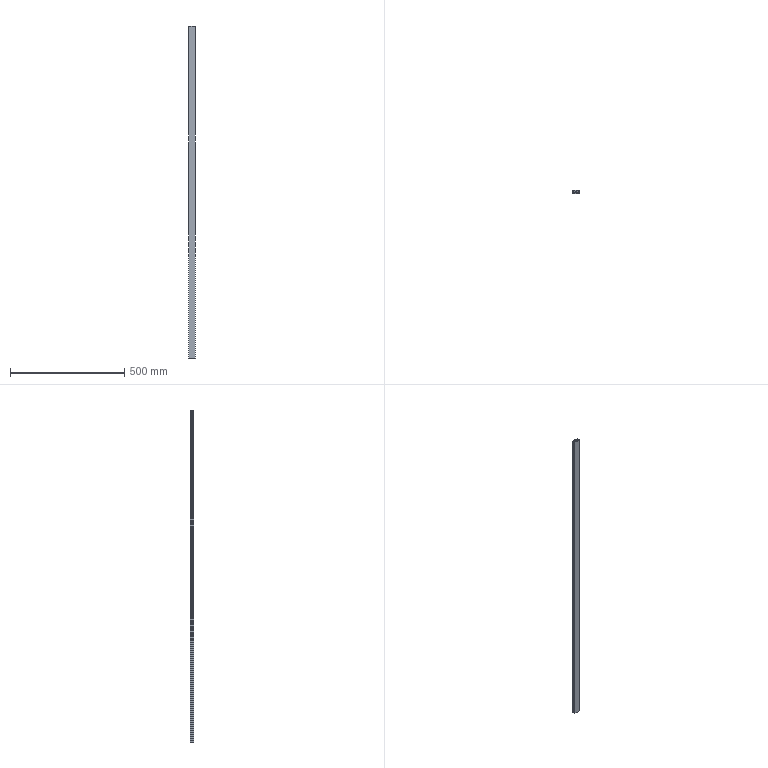Part | SolidWorks | features BaseBody 1, HoleWzd 1, MoveFace 1 | 1 solid | 53 faces | box 30 x 15 x 1456 mm | volume 351142 mm3 | plane 38 | cylinder 15 | commonest cylinder face diameters 1 x6 5 x5 2 x4